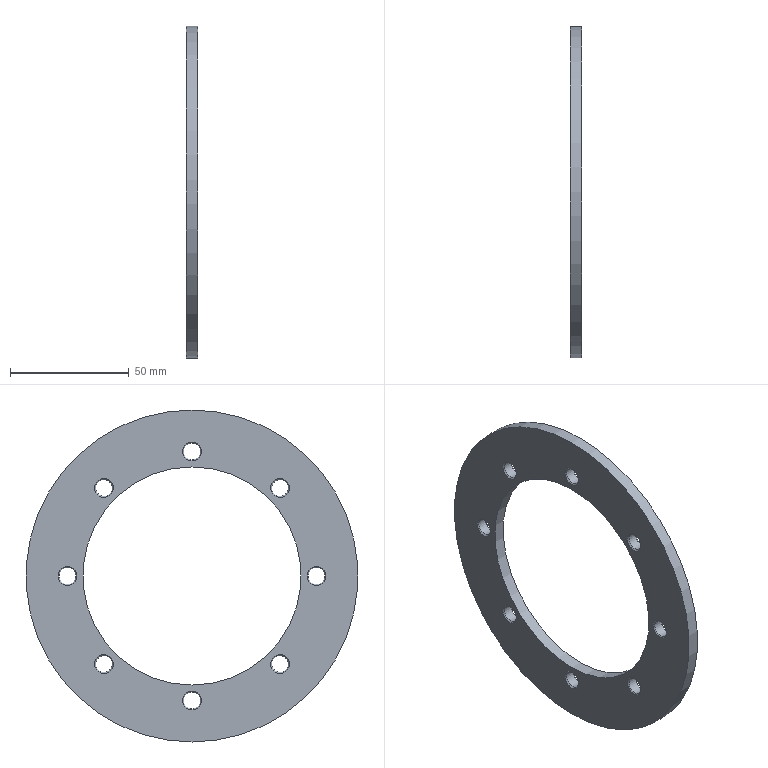Part | STEP file | Brake stopper | 1 solid | 28 faces | box 5 x 140 x 140 mm | volume 42146 mm3 | cone 16 | cylinder 10 | plane 2 | commonest cylinder face diameters 7 x8 92 x1 140 x1
STEP:
#1=CARTESIAN_POINT('',(0.,0.,-70.));
#2=VERTEX_POINT('',#1);
#3=CARTESIAN_POINT('',(0.,0.,0.));
#4=DIRECTION('',(1.,0.,0.));
#5=DIRECTION('',(0.,0.,-1.));
#6=AXIS2_PLACEMENT_3D('',#3,#4,#5);
#7=CIRCLE('',#6,70.);
#8=EDGE_CURVE('',#2,#2,#7,.T.);
#9=ORIENTED_EDGE('',*,*,#8,.F.);
#10=EDGE_LOOP('',(#9));
#11=FACE_BOUND('',#10,.T.);
#12=CARTESIAN_POINT('',(0.,39.952,34.295));
#13=VERTEX_POINT('',#12);
#14=CARTESIAN_POINT('',(0.,37.123,37.123));
#15=DIRECTION('',(-1.,0.,0.));
#16=DIRECTION('',(0.,0.7071,-0.7071));
#17=AXIS2_PLACEMENT_3D('',#14,#15,#16);
#18=CIRCLE('',#17,4.);
#19=EDGE_CURVE('',#13,#13,#18,.F.);
#20=ORIENTED_EDGE('',*,*,#19,.T.);
#21=EDGE_LOOP('',(#20));
#22=FACE_BOUND('',#21,.T.);
#23=CARTESIAN_POINT('',(0.,34.295,-39.952));
#24=VERTEX_POINT('',#23);
#25=CARTESIAN_POINT('',(0.,37.123,-37.123));
#26=DIRECTION('',(-1.,0.,0.));
#27=DIRECTION('',(0.,-0.7071,-0.7071));
#28=AXIS2_PLACEMENT_3D('',#25,#26,#27);
#29=CIRCLE('',#28,4.);
#30=EDGE_CURVE('',#24,#24,#29,.F.);
#31=ORIENTED_EDGE('',*,*,#30,.T.);
#32=EDGE_LOOP('',(#31));
#33=FACE_BOUND('',#32,.T.);
#34=CARTESIAN_POINT('',(0.,-39.952,-34.295));
#35=VERTEX_POINT('',#34);
#36=CARTESIAN_POINT('',(0.,-37.123,-37.123));
#37=DIRECTION('',(-1.,0.,0.));
#38=DIRECTION('',(0.,-0.7071,0.7071));
#39=AXIS2_PLACEMENT_3D('',#36,#37,#38);
#40=CIRCLE('',#39,4.);
#41=EDGE_CURVE('',#35,#35,#40,.F.);
#42=ORIENTED_EDGE('',*,*,#41,.T.);
#43=EDGE_LOOP('',(#42));
#44=FACE_BOUND('',#43,.T.);
#45=CARTESIAN_POINT('',(0.,-34.295,39.952));
#46=VERTEX_POINT('',#45);
#47=CARTESIAN_POINT('',(0.,-37.123,37.123));
#48=DIRECTION('',(-1.,0.,0.));
#49=DIRECTION('',(0.,0.7071,0.7071));
#50=AXIS2_PLACEMENT_3D('',#47,#48,#49);
#51=CIRCLE('',#50,4.);
#52=EDGE_CURVE('',#46,#46,#51,.F.);
#53=ORIENTED_EDGE('',*,*,#52,.T.);
#54=EDGE_LOOP('',(#53));
#55=FACE_BOUND('',#54,.T.);
#56=CARTESIAN_POINT('',(0.,4.,52.5));
#57=VERTEX_POINT('',#56);
#58=CARTESIAN_POINT('',(0.,0.,52.5));
#59=DIRECTION('',(-1.,0.,0.));
#60=DIRECTION('',(0.,1.,0.));
#61=AXIS2_PLACEMENT_3D('',#58,#59,#60);
#62=CIRCLE('',#61,4.);
#63=EDGE_CURVE('',#57,#57,#62,.F.);
#64=ORIENTED_EDGE('',*,*,#63,.T.);
#65=EDGE_LOOP('',(#64));
#66=FACE_BOUND('',#65,.T.);
#67=CARTESIAN_POINT('',(0.,0.,-46.));
#68=VERTEX_POINT('',#67);
#69=CARTESIAN_POINT('',(0.,0.,0.));
#70=DIRECTION('',(1.,0.,0.));
#71=DIRECTION('',(0.,0.,-1.));
#72=AXIS2_PLACEMENT_3D('',#69,#70,#71);
#73=CIRCLE('',#72,46.);
#74=EDGE_CURVE('',#68,#68,#73,.T.);
#75=ORIENTED_EDGE('',*,*,#74,.T.);
#76=EDGE_LOOP('',(#75));
#77=FACE_BOUND('',#76,.T.);
#78=CARTESIAN_POINT('',(0.,-52.5,4.));
#79=VERTEX_POINT('',#78);
#80=CARTESIAN_POINT('',(0.,-52.5,0.));
#81=DIRECTION('',(-1.,0.,0.));
#82=DIRECTION('',(0.,0.,1.));
#83=AXIS2_PLACEMENT_3D('',#80,#81,#82);
#84=CIRCLE('',#83,4.);
#85=EDGE_CURVE('',#79,#79,#84,.F.);
#86=ORIENTED_EDGE('',*,*,#85,.T.);
#87=EDGE_LOOP('',(#86));
#88=FACE_BOUND('',#87,.T.);
#89=CARTESIAN_POINT('',(0.,-4.,-52.5));
#90=VERTEX_POINT('',#89);
#91=CARTESIAN_POINT('',(0.,0.,-52.5));
#92=DIRECTION('',(-1.,0.,0.));
#93=DIRECTION('',(0.,-1.,0.));
#94=AXIS2_PLACEMENT_3D('',#91,#92,#93);
#95=CIRCLE('',#94,4.);
#96=EDGE_CURVE('',#90,#90,#95,.F.);
#97=ORIENTED_EDGE('',*,*,#96,.T.);
#98=EDGE_LOOP('',(#97));
#99=FACE_BOUND('',#98,.T.);
#100=CARTESIAN_POINT('',(0.,52.5,-4.));
#101=VERTEX_POINT('',#100);
#102=CARTESIAN_POINT('',(0.,52.5,0.));
#103=DIRECTION('',(-1.,0.,0.));
#104=DIRECTION('',(0.,0.,-1.));
#105=AXIS2_PLACEMENT_3D('',#102,#103,#104);
#106=CIRCLE('',#105,4.);
#107=EDGE_CURVE('',#101,#101,#106,.F.);
#108=ORIENTED_EDGE('',*,*,#107,.T.);
#109=EDGE_LOOP('',(#108));
#110=FACE_BOUND('',#109,.T.);
#111=CARTESIAN_POINT('',(0.,0.,0.));
#112=DIRECTION('',(1.,0.,0.));
#113=DIRECTION('',(0.,0.,-1.));
#114=AXIS2_PLACEMENT_3D('',#111,#112,#113);
#115=PLANE('',#114);
#116=ADVANCED_FACE('',(#11,#22,#33,#44,#55,#66,#77,#88,#99,#110),#115,.F.);
#117=CARTESIAN_POINT('',(5.,0.,-70.));
#118=VERTEX_POINT('',#117);
#119=CARTESIAN_POINT('',(5.,0.,0.));
#120=DIRECTION('',(1.,0.,0.));
#121=DIRECTION('',(0.,0.,-1.));
#122=AXIS2_PLACEMENT_3D('',#119,#120,#121);
#123=CIRCLE('',#122,70.);
#124=EDGE_CURVE('',#118,#118,#123,.T.);
#125=ORIENTED_EDGE('',*,*,#124,.T.);
#126=EDGE_LOOP('',(#125));
#127=FACE_BOUND('',#126,.T.);
#128=CARTESIAN_POINT('',(5.,39.952,34.295));
#129=VERTEX_POINT('',#128);
#130=CARTESIAN_POINT('',(5.,37.123,37.123));
#131=DIRECTION('',(-1.,0.,0.));
#132=DIRECTION('',(0.,0.7071,-0.7071));
#133=AXIS2_PLACEMENT_3D('',#130,#131,#132);
#134=CIRCLE('',#133,4.);
#135=EDGE_CURVE('',#129,#129,#134,.T.);
#136=ORIENTED_EDGE('',*,*,#135,.T.);
#137=EDGE_LOOP('',(#136));
#138=FACE_BOUND('',#137,.T.);
#139=CARTESIAN_POINT('',(5.,34.295,-39.952));
#140=VERTEX_POINT('',#139);
#141=CARTESIAN_POINT('',(5.,37.123,-37.123));
#142=DIRECTION('',(-1.,0.,0.));
#143=DIRECTION('',(0.,-0.7071,-0.7071));
#144=AXIS2_PLACEMENT_3D('',#141,#142,#143);
#145=CIRCLE('',#144,4.);
#146=EDGE_CURVE('',#140,#140,#145,.T.);
#147=ORIENTED_EDGE('',*,*,#146,.T.);
#148=EDGE_LOOP('',(#147));
#149=FACE_BOUND('',#148,.T.);
#150=CARTESIAN_POINT('',(5.,-39.952,-34.295));
#151=VERTEX_POINT('',#150);
#152=CARTESIAN_POINT('',(5.,-37.123,-37.123));
#153=DIRECTION('',(-1.,0.,0.));
#154=DIRECTION('',(0.,-0.7071,0.7071));
#155=AXIS2_PLACEMENT_3D('',#152,#153,#154);
#156=CIRCLE('',#155,4.);
#157=EDGE_CURVE('',#151,#151,#156,.T.);
#158=ORIENTED_EDGE('',*,*,#157,.T.);
#159=EDGE_LOOP('',(#158));
#160=FACE_BOUND('',#159,.T.);
#161=CARTESIAN_POINT('',(5.,-34.295,39.952));
#162=VERTEX_POINT('',#161);
#163=CARTESIAN_POINT('',(5.,-37.123,37.123));
#164=DIRECTION('',(-1.,0.,0.));
#165=DIRECTION('',(0.,0.7071,0.7071));
#166=AXIS2_PLACEMENT_3D('',#163,#164,#165);
#167=CIRCLE('',#166,4.);
#168=EDGE_CURVE('',#162,#162,#167,.T.);
#169=ORIENTED_EDGE('',*,*,#168,.T.);
#170=EDGE_LOOP('',(#169));
#171=FACE_BOUND('',#170,.T.);
#172=CARTESIAN_POINT('',(5.,4.,52.5));
#173=VERTEX_POINT('',#172);
#174=CARTESIAN_POINT('',(5.,0.,52.5));
#175=DIRECTION('',(-1.,0.,0.));
#176=DIRECTION('',(0.,1.,0.));
#177=AXIS2_PLACEMENT_3D('',#174,#175,#176);
#178=CIRCLE('',#177,4.);
#179=EDGE_CURVE('',#173,#173,#178,.T.);
#180=ORIENTED_EDGE('',*,*,#179,.T.);
#181=EDGE_LOOP('',(#180));
#182=FACE_BOUND('',#181,.T.);
#183=CARTESIAN_POINT('',(5.,0.,-46.));
#184=VERTEX_POINT('',#183);
#185=CARTESIAN_POINT('',(5.,0.,0.));
#186=DIRECTION('',(1.,0.,0.));
#187=DIRECTION('',(0.,0.,-1.));
#188=AXIS2_PLACEMENT_3D('',#185,#186,#187);
#189=CIRCLE('',#188,46.);
#190=EDGE_CURVE('',#184,#184,#189,.F.);
#191=ORIENTED_EDGE('',*,*,#190,.T.);
#192=EDGE_LOOP('',(#191));
#193=FACE_BOUND('',#192,.T.);
#194=CARTESIAN_POINT('',(5.,-52.5,4.));
#195=VERTEX_POINT('',#194);
#196=CARTESIAN_POINT('',(5.,-52.5,0.));
#197=DIRECTION('',(-1.,0.,0.));
#198=DIRECTION('',(0.,0.,1.));
#199=AXIS2_PLACEMENT_3D('',#196,#197,#198);
#200=CIRCLE('',#199,4.);
#201=EDGE_CURVE('',#195,#195,#200,.T.);
#202=ORIENTED_EDGE('',*,*,#201,.T.);
#203=EDGE_LOOP('',(#202));
#204=FACE_BOUND('',#203,.T.);
#205=CARTESIAN_POINT('',(5.,-4.,-52.5));
#206=VERTEX_POINT('',#205);
#207=CARTESIAN_POINT('',(5.,0.,-52.5));
#208=DIRECTION('',(-1.,0.,0.));
#209=DIRECTION('',(0.,-1.,0.));
#210=AXIS2_PLACEMENT_3D('',#207,#208,#209);
#211=CIRCLE('',#210,4.);
#212=EDGE_CURVE('',#206,#206,#211,.T.);
#213=ORIENTED_EDGE('',*,*,#212,.T.);
#214=EDGE_LOOP('',(#213));
#215=FACE_BOUND('',#214,.T.);
#216=CARTESIAN_POINT('',(5.,52.5,-4.));
#217=VERTEX_POINT('',#216);
#218=CARTESIAN_POINT('',(5.,52.5,0.));
#219=DIRECTION('',(-1.,0.,0.));
#220=DIRECTION('',(0.,0.,-1.));
#221=AXIS2_PLACEMENT_3D('',#218,#219,#220);
#222=CIRCLE('',#221,4.);
#223=EDGE_CURVE('',#217,#217,#222,.T.);
#224=ORIENTED_EDGE('',*,*,#223,.T.);
#225=EDGE_LOOP('',(#224));
#226=FACE_BOUND('',#225,.T.);
#227=CARTESIAN_POINT('',(5.,0.,0.));
#228=DIRECTION('',(1.,0.,0.));
#229=DIRECTION('',(0.,0.,-1.));
#230=AXIS2_PLACEMENT_3D('',#227,#228,#229);
#231=PLANE('',#230);
#232=ADVANCED_FACE('',(#127,#138,#149,#160,#171,#182,#193,#204,#215,#226),#231,.T.);
#233=CARTESIAN_POINT('',(4.5,39.598,34.648));
#234=VERTEX_POINT('',#233);
#235=CARTESIAN_POINT('',(4.5,37.123,37.123));
#236=DIRECTION('',(-1.,0.,0.));
#237=DIRECTION('',(0.,0.7071,-0.7071));
#238=AXIS2_PLACEMENT_3D('',#235,#236,#237);
#239=CIRCLE('',#238,3.5);
#240=EDGE_CURVE('',#234,#234,#239,.T.);
#241=ORIENTED_EDGE('',*,*,#240,.F.);
#242=EDGE_LOOP('',(#241));
#243=FACE_OUTER_BOUND('',#242,.T.);
#244=CARTESIAN_POINT('',(0.5,39.598,34.648));
#245=VERTEX_POINT('',#244);
#246=CARTESIAN_POINT('',(0.5,37.123,37.123));
#247=DIRECTION('',(-1.,0.,0.));
#248=DIRECTION('',(0.,0.7071,-0.7071));
#249=AXIS2_PLACEMENT_3D('',#246,#247,#248);
#250=CIRCLE('',#249,3.5);
#251=EDGE_CURVE('',#245,#245,#250,.F.);
#252=ORIENTED_EDGE('',*,*,#251,.F.);
#253=EDGE_LOOP('',(#252));
#254=FACE_OUTER_BOUND('',#253,.T.);
#255=CARTESIAN_POINT('',(40.,37.123,37.123));
#256=DIRECTION('',(-1.,0.,0.));
#257=DIRECTION('',(0.,0.7071,-0.7071));
#258=AXIS2_PLACEMENT_3D('',#255,#256,#257);
#259=CYLINDRICAL_SURFACE('',#258,3.5);
#260=ADVANCED_FACE('',(#243,#254),#259,.F.);
#261=CARTESIAN_POINT('',(4.5,52.5,-3.5));
#262=VERTEX_POINT('',#261);
#263=CARTESIAN_POINT('',(4.5,52.5,0.));
#264=DIRECTION('',(-1.,0.,0.));
#265=DIRECTION('',(0.,0.,-1.));
#266=AXIS2_PLACEMENT_3D('',#263,#264,#265);
#267=CIRCLE('',#266,3.5);
#268=EDGE_CURVE('',#262,#262,#267,.T.);
#269=ORIENTED_EDGE('',*,*,#268,.F.);
#270=EDGE_LOOP('',(#269));
#271=FACE_OUTER_BOUND('',#270,.T.);
#272=CARTESIAN_POINT('',(0.5,52.5,-3.5));
#273=VERTEX_POINT('',#272);
#274=CARTESIAN_POINT('',(0.5,52.5,0.));
#275=DIRECTION('',(-1.,0.,0.));
#276=DIRECTION('',(0.,0.,-1.));
#277=AXIS2_PLACEMENT_3D('',#274,#275,#276);
#278=CIRCLE('',#277,3.5);
#279=EDGE_CURVE('',#273,#273,#278,.F.);
#280=ORIENTED_EDGE('',*,*,#279,.F.);
#281=EDGE_LOOP('',(#280));
#282=FACE_OUTER_BOUND('',#281,.T.);
#283=CARTESIAN_POINT('',(40.,52.5,0.));
#284=DIRECTION('',(-1.,0.,0.));
#285=DIRECTION('',(0.,0.,-1.));
#286=AXIS2_PLACEMENT_3D('',#283,#284,#285);
#287=CYLINDRICAL_SURFACE('',#286,3.5);
#288=ADVANCED_FACE('',(#271,#282),#287,.F.);
#289=CARTESIAN_POINT('',(4.5,34.648,-39.598));
#290=VERTEX_POINT('',#289);
#291=CARTESIAN_POINT('',(4.5,37.123,-37.123));
#292=DIRECTION('',(-1.,0.,0.));
#293=DIRECTION('',(0.,-0.7071,-0.7071));
#294=AXIS2_PLACEMENT_3D('',#291,#292,#293);
#295=CIRCLE('',#294,3.5);
#296=EDGE_CURVE('',#290,#290,#295,.T.);
#297=ORIENTED_EDGE('',*,*,#296,.F.);
#298=EDGE_LOOP('',(#297));
#299=FACE_OUTER_BOUND('',#298,.T.);
#300=CARTESIAN_POINT('',(0.5,34.648,-39.598));
#301=VERTEX_POINT('',#300);
#302=CARTESIAN_POINT('',(0.5,37.123,-37.123));
#303=DIRECTION('',(-1.,0.,0.));
#304=DIRECTION('',(0.,-0.7071,-0.7071));
#305=AXIS2_PLACEMENT_3D('',#302,#303,#304);
#306=CIRCLE('',#305,3.5);
#307=EDGE_CURVE('',#301,#301,#306,.F.);
#308=ORIENTED_EDGE('',*,*,#307,.F.);
#309=EDGE_LOOP('',(#308));
#310=FACE_OUTER_BOUND('',#309,.T.);
#311=CARTESIAN_POINT('',(40.,37.123,-37.123));
#312=DIRECTION('',(-1.,0.,0.));
#313=DIRECTION('',(0.,-0.7071,-0.7071));
#314=AXIS2_PLACEMENT_3D('',#311,#312,#313);
#315=CYLINDRICAL_SURFACE('',#314,3.5);
#316=ADVANCED_FACE('',(#299,#310),#315,.F.);
#317=CARTESIAN_POINT('',(4.5,-3.5,-52.5));
#318=VERTEX_POINT('',#317);
#319=CARTESIAN_POINT('',(4.5,0.,-52.5));
#320=DIRECTION('',(-1.,0.,0.));
#321=DIRECTION('',(0.,-1.,0.));
#322=AXIS2_PLACEMENT_3D('',#319,#320,#321);
#323=CIRCLE('',#322,3.5);
#324=EDGE_CURVE('',#318,#318,#323,.T.);
#325=ORIENTED_EDGE('',*,*,#324,.F.);
#326=EDGE_LOOP('',(#325));
#327=FACE_OUTER_BOUND('',#326,.T.);
#328=CARTESIAN_POINT('',(0.5,-3.5,-52.5));
#329=VERTEX_POINT('',#328);
#330=CARTESIAN_POINT('',(0.5,0.,-52.5));
#331=DIRECTION('',(-1.,0.,0.));
#332=DIRECTION('',(0.,-1.,0.));
#333=AXIS2_PLACEMENT_3D('',#330,#331,#332);
#334=CIRCLE('',#333,3.5);
#335=EDGE_CURVE('',#329,#329,#334,.F.);
#336=ORIENTED_EDGE('',*,*,#335,.F.);
#337=EDGE_LOOP('',(#336));
#338=FACE_OUTER_BOUND('',#337,.T.);
#339=CARTESIAN_POINT('',(40.,0.,-52.5));
#340=DIRECTION('',(-1.,0.,0.));
#341=DIRECTION('',(0.,-1.,0.));
#342=AXIS2_PLACEMENT_3D('',#339,#340,#341);
#343=CYLINDRICAL_SURFACE('',#342,3.5);
#344=ADVANCED_FACE('',(#327,#338),#343,.F.);
#345=CARTESIAN_POINT('',(4.5,-39.598,-34.648));
#346=VERTEX_POINT('',#345);
#347=CARTESIAN_POINT('',(4.5,-37.123,-37.123));
#348=DIRECTION('',(-1.,0.,0.));
#349=DIRECTION('',(0.,-0.7071,0.7071));
#350=AXIS2_PLACEMENT_3D('',#347,#348,#349);
#351=CIRCLE('',#350,3.5);
#352=EDGE_CURVE('',#346,#346,#351,.T.);
#353=ORIENTED_EDGE('',*,*,#352,.F.);
#354=EDGE_LOOP('',(#353));
#355=FACE_OUTER_BOUND('',#354,.T.);
#356=CARTESIAN_POINT('',(0.5,-39.598,-34.648));
#357=VERTEX_POINT('',#356);
#358=CARTESIAN_POINT('',(0.5,-37.123,-37.123));
#359=DIRECTION('',(-1.,0.,0.));
#360=DIRECTION('',(0.,-0.7071,0.7071));
#361=AXIS2_PLACEMENT_3D('',#358,#359,#360);
#362=CIRCLE('',#361,3.5);
#363=EDGE_CURVE('',#357,#357,#362,.F.);
#364=ORIENTED_EDGE('',*,*,#363,.F.);
#365=EDGE_LOOP('',(#364));
#366=FACE_OUTER_BOUND('',#365,.T.);
#367=CARTESIAN_POINT('',(40.,-37.123,-37.123));
#368=DIRECTION('',(-1.,0.,0.));
#369=DIRECTION('',(0.,-0.7071,0.7071));
#370=AXIS2_PLACEMENT_3D('',#367,#368,#369);
#371=CYLINDRICAL_SURFACE('',#370,3.5);
#372=ADVANCED_FACE('',(#355,#366),#371,.F.);
#373=CARTESIAN_POINT('',(4.5,-52.5,3.5));
#374=VERTEX_POINT('',#373);
#375=CARTESIAN_POINT('',(4.5,-52.5,0.));
#376=DIRECTION('',(-1.,0.,0.));
#377=DIRECTION('',(0.,0.,1.));
#378=AXIS2_PLACEMENT_3D('',#375,#376,#377);
#379=CIRCLE('',#378,3.5);
#380=EDGE_CURVE('',#374,#374,#379,.T.);
#381=ORIENTED_EDGE('',*,*,#380,.F.);
#382=EDGE_LOOP('',(#381));
#383=FACE_OUTER_BOUND('',#382,.T.);
#384=CARTESIAN_POINT('',(0.5,-52.5,3.5));
#385=VERTEX_POINT('',#384);
#386=CARTESIAN_POINT('',(0.5,-52.5,0.));
#387=DIRECTION('',(-1.,0.,0.));
#388=DIRECTION('',(0.,0.,1.));
#389=AXIS2_PLACEMENT_3D('',#386,#387,#388);
#390=CIRCLE('',#389,3.5);
#391=EDGE_CURVE('',#385,#385,#390,.F.);
#392=ORIENTED_EDGE('',*,*,#391,.F.);
#393=EDGE_LOOP('',(#392));
#394=FACE_OUTER_BOUND('',#393,.T.);
#395=CARTESIAN_POINT('',(40.,-52.5,0.));
#396=DIRECTION('',(-1.,0.,0.));
#397=DIRECTION('',(0.,0.,1.));
#398=AXIS2_PLACEMENT_3D('',#395,#396,#397);
#399=CYLINDRICAL_SURFACE('',#398,3.5);
#400=ADVANCED_FACE('',(#383,#394),#399,.F.);
#401=CARTESIAN_POINT('',(4.5,-34.648,39.598));
#402=VERTEX_POINT('',#401);
#403=CARTESIAN_POINT('',(4.5,-37.123,37.123));
#404=DIRECTION('',(-1.,0.,0.));
#405=DIRECTION('',(0.,0.7071,0.7071));
#406=AXIS2_PLACEMENT_3D('',#403,#404,#405);
#407=CIRCLE('',#406,3.5);
#408=EDGE_CURVE('',#402,#402,#407,.T.);
#409=ORIENTED_EDGE('',*,*,#408,.F.);
#410=EDGE_LOOP('',(#409));
#411=FACE_OUTER_BOUND('',#410,.T.);
#412=CARTESIAN_POINT('',(0.5,-34.648,39.598));
#413=VERTEX_POINT('',#412);
#414=CARTESIAN_POINT('',(0.5,-37.123,37.123));
#415=DIRECTION('',(-1.,0.,0.));
#416=DIRECTION('',(0.,0.7071,0.7071));
#417=AXIS2_PLACEMENT_3D('',#414,#415,#416);
#418=CIRCLE('',#417,3.5);
#419=EDGE_CURVE('',#413,#413,#418,.F.);
#420=ORIENTED_EDGE('',*,*,#419,.F.);
#421=EDGE_LOOP('',(#420));
#422=FACE_OUTER_BOUND('',#421,.T.);
#423=CARTESIAN_POINT('',(40.,-37.123,37.123));
#424=DIRECTION('',(-1.,0.,0.));
#425=DIRECTION('',(0.,0.7071,0.7071));
#426=AXIS2_PLACEMENT_3D('',#423,#424,#425);
#427=CYLINDRICAL_SURFACE('',#426,3.5);
#428=ADVANCED_FACE('',(#411,#422),#427,.F.);
#429=ORIENTED_EDGE('',*,*,#124,.F.);
#430=EDGE_LOOP('',(#429));
#431=FACE_OUTER_BOUND('',#430,.T.);
#432=ORIENTED_EDGE('',*,*,#8,.T.);
#433=EDGE_LOOP('',(#432));
#434=FACE_OUTER_BOUND('',#433,.T.);
#435=CARTESIAN_POINT('',(0.,0.,0.));
#436=DIRECTION('',(1.,0.,0.));
#437=DIRECTION('',(0.,0.,-1.));
#438=AXIS2_PLACEMENT_3D('',#435,#436,#437);
#439=CYLINDRICAL_SURFACE('',#438,70.);
#440=ADVANCED_FACE('',(#431,#434),#439,.T.);
#441=ORIENTED_EDGE('',*,*,#190,.F.);
#442=EDGE_LOOP('',(#441));
#443=FACE_OUTER_BOUND('',#442,.T.);
#444=ORIENTED_EDGE('',*,*,#74,.F.);
#445=EDGE_LOOP('',(#444));
#446=FACE_OUTER_BOUND('',#445,.T.);
#447=CARTESIAN_POINT('',(0.,0.,0.));
#448=DIRECTION('',(1.,0.,0.));
#449=DIRECTION('',(0.,0.,-1.));
#450=AXIS2_PLACEMENT_3D('',#447,#448,#449);
#451=CYLINDRICAL_SURFACE('',#450,46.);
#452=ADVANCED_FACE('',(#443,#446),#451,.F.);
#453=CARTESIAN_POINT('',(0.5,3.5,52.5));
#454=VERTEX_POINT('',#453);
#455=CARTESIAN_POINT('',(0.5,0.,52.5));
#456=DIRECTION('',(-1.,0.,0.));
#457=DIRECTION('',(0.,1.,0.));
#458=AXIS2_PLACEMENT_3D('',#455,#456,#457);
#459=CIRCLE('',#458,3.5);
#460=EDGE_CURVE('',#454,#454,#459,.F.);
#461=ORIENTED_EDGE('',*,*,#460,.T.);
#462=EDGE_LOOP('',(#461));
#463=FACE_OUTER_BOUND('',#462,.T.);
#464=ORIENTED_EDGE('',*,*,#63,.F.);
#465=EDGE_LOOP('',(#464));
#466=FACE_OUTER_BOUND('',#465,.T.);
#467=CARTESIAN_POINT('',(0.25,0.,52.5));
#468=DIRECTION('',(-1.,0.,0.));
#469=DIRECTION('',(0.,1.,0.));
#470=AXIS2_PLACEMENT_3D('',#467,#468,#469);
#471=CONICAL_SURFACE('',#470,3.75,0.7854);
#472=ADVANCED_FACE('',(#463,#466),#471,.F.);
#473=ORIENTED_EDGE('',*,*,#179,.F.);
#474=EDGE_LOOP('',(#473));
#475=FACE_OUTER_BOUND('',#474,.T.);
#476=CARTESIAN_POINT('',(4.5,3.5,52.5));
#477=VERTEX_POINT('',#476);
#478=CARTESIAN_POINT('',(4.5,0.,52.5));
#479=DIRECTION('',(-1.,0.,0.));
#480=DIRECTION('',(0.,1.,0.));
#481=AXIS2_PLACEMENT_3D('',#478,#479,#480);
#482=CIRCLE('',#481,3.5);
#483=EDGE_CURVE('',#477,#477,#482,.T.);
#484=ORIENTED_EDGE('',*,*,#483,.T.);
#485=EDGE_LOOP('',(#484));
#486=FACE_OUTER_BOUND('',#485,.T.);
#487=CARTESIAN_POINT('',(4.75,0.,52.5));
#488=DIRECTION('',(1.,0.,0.));
#489=DIRECTION('',(0.,-1.,0.));
#490=AXIS2_PLACEMENT_3D('',#487,#488,#489);
#491=CONICAL_SURFACE('',#490,3.75,0.7854);
#492=ADVANCED_FACE('',(#475,#486),#491,.F.);
#493=ORIENTED_EDGE('',*,*,#483,.F.);
#494=EDGE_LOOP('',(#493));
#495=FACE_OUTER_BOUND('',#494,.T.);
#496=ORIENTED_EDGE('',*,*,#460,.F.);
#497=EDGE_LOOP('',(#496));
#498=FACE_OUTER_BOUND('',#497,.T.);
#499=CARTESIAN_POINT('',(40.,0.,52.5));
#500=DIRECTION('',(-1.,0.,0.));
#501=DIRECTION('',(0.,1.,0.));
#502=AXIS2_PLACEMENT_3D('',#499,#500,#501);
#503=CYLINDRICAL_SURFACE('',#502,3.5);
#504=ADVANCED_FACE('',(#495,#498),#503,.F.);
#505=ORIENTED_EDGE('',*,*,#419,.T.);
#506=EDGE_LOOP('',(#505));
#507=FACE_OUTER_BOUND('',#506,.T.);
#508=ORIENTED_EDGE('',*,*,#52,.F.);
#509=EDGE_LOOP('',(#508));
#510=FACE_OUTER_BOUND('',#509,.T.);
#511=CARTESIAN_POINT('',(0.25,-37.123,37.123));
#512=DIRECTION('',(-1.,0.,0.));
#513=DIRECTION('',(0.,0.7071,0.7071));
#514=AXIS2_PLACEMENT_3D('',#511,#512,#513);
#515=CONICAL_SURFACE('',#514,3.75,0.7854);
#516=ADVANCED_FACE('',(#507,#510),#515,.F.);
#517=ORIENTED_EDGE('',*,*,#168,.F.);
#518=EDGE_LOOP('',(#517));
#519=FACE_OUTER_BOUND('',#518,.T.);
#520=ORIENTED_EDGE('',*,*,#408,.T.);
#521=EDGE_LOOP('',(#520));
#522=FACE_OUTER_BOUND('',#521,.T.);
#523=CARTESIAN_POINT('',(4.75,-37.123,37.123));
#524=DIRECTION('',(1.,0.,0.));
#525=DIRECTION('',(0.,-0.7071,-0.7071));
#526=AXIS2_PLACEMENT_3D('',#523,#524,#525);
#527=CONICAL_SURFACE('',#526,3.75,0.7854);
#528=ADVANCED_FACE('',(#519,#522),#527,.F.);
#529=ORIENTED_EDGE('',*,*,#391,.T.);
#530=EDGE_LOOP('',(#529));
#531=FACE_OUTER_BOUND('',#530,.T.);
#532=ORIENTED_EDGE('',*,*,#85,.F.);
#533=EDGE_LOOP('',(#532));
#534=FACE_OUTER_BOUND('',#533,.T.);
#535=CARTESIAN_POINT('',(0.25,-52.5,0.));
#536=DIRECTION('',(-1.,0.,0.));
#537=DIRECTION('',(0.,0.,1.));
#538=AXIS2_PLACEMENT_3D('',#535,#536,#537);
#539=CONICAL_SURFACE('',#538,3.75,0.7854);
#540=ADVANCED_FACE('',(#531,#534),#539,.F.);
#541=ORIENTED_EDGE('',*,*,#201,.F.);
#542=EDGE_LOOP('',(#541));
#543=FACE_OUTER_BOUND('',#542,.T.);
#544=ORIENTED_EDGE('',*,*,#380,.T.);
#545=EDGE_LOOP('',(#544));
#546=FACE_OUTER_BOUND('',#545,.T.);
#547=CARTESIAN_POINT('',(4.75,-52.5,0.));
#548=DIRECTION('',(1.,0.,0.));
#549=DIRECTION('',(0.,0.,-1.));
#550=AXIS2_PLACEMENT_3D('',#547,#548,#549);
#551=CONICAL_SURFACE('',#550,3.75,0.7854);
#552=ADVANCED_FACE('',(#543,#546),#551,.F.);
#553=ORIENTED_EDGE('',*,*,#363,.T.);
#554=EDGE_LOOP('',(#553));
#555=FACE_OUTER_BOUND('',#554,.T.);
#556=ORIENTED_EDGE('',*,*,#41,.F.);
#557=EDGE_LOOP('',(#556));
#558=FACE_OUTER_BOUND('',#557,.T.);
#559=CARTESIAN_POINT('',(0.25,-37.123,-37.123));
#560=DIRECTION('',(-1.,0.,0.));
#561=DIRECTION('',(0.,-0.7071,0.7071));
#562=AXIS2_PLACEMENT_3D('',#559,#560,#561);
#563=CONICAL_SURFACE('',#562,3.75,0.7854);
#564=ADVANCED_FACE('',(#555,#558),#563,.F.);
#565=ORIENTED_EDGE('',*,*,#157,.F.);
#566=EDGE_LOOP('',(#565));
#567=FACE_OUTER_BOUND('',#566,.T.);
#568=ORIENTED_EDGE('',*,*,#352,.T.);
#569=EDGE_LOOP('',(#568));
#570=FACE_OUTER_BOUND('',#569,.T.);
#571=CARTESIAN_POINT('',(4.75,-37.123,-37.123));
#572=DIRECTION('',(1.,0.,0.));
#573=DIRECTION('',(0.,0.7071,-0.7071));
#574=AXIS2_PLACEMENT_3D('',#571,#572,#573);
#575=CONICAL_SURFACE('',#574,3.75,0.7854);
#576=ADVANCED_FACE('',(#567,#570),#575,.F.);
#577=ORIENTED_EDGE('',*,*,#335,.T.);
#578=EDGE_LOOP('',(#577));
#579=FACE_OUTER_BOUND('',#578,.T.);
#580=ORIENTED_EDGE('',*,*,#96,.F.);
#581=EDGE_LOOP('',(#580));
#582=FACE_OUTER_BOUND('',#581,.T.);
#583=CARTESIAN_POINT('',(0.25,0.,-52.5));
#584=DIRECTION('',(-1.,0.,0.));
#585=DIRECTION('',(0.,-1.,0.));
#586=AXIS2_PLACEMENT_3D('',#583,#584,#585);
#587=CONICAL_SURFACE('',#586,3.75,0.7854);
#588=ADVANCED_FACE('',(#579,#582),#587,.F.);
#589=ORIENTED_EDGE('',*,*,#212,.F.);
#590=EDGE_LOOP('',(#589));
#591=FACE_OUTER_BOUND('',#590,.T.);
#592=ORIENTED_EDGE('',*,*,#324,.T.);
#593=EDGE_LOOP('',(#592));
#594=FACE_OUTER_BOUND('',#593,.T.);
#595=CARTESIAN_POINT('',(4.75,0.,-52.5));
#596=DIRECTION('',(1.,0.,0.));
#597=DIRECTION('',(0.,1.,0.));
#598=AXIS2_PLACEMENT_3D('',#595,#596,#597);
#599=CONICAL_SURFACE('',#598,3.75,0.7854);
#600=ADVANCED_FACE('',(#591,#594),#599,.F.);
#601=ORIENTED_EDGE('',*,*,#307,.T.);
#602=EDGE_LOOP('',(#601));
#603=FACE_OUTER_BOUND('',#602,.T.);
#604=ORIENTED_EDGE('',*,*,#30,.F.);
#605=EDGE_LOOP('',(#604));
#606=FACE_OUTER_BOUND('',#605,.T.);
#607=CARTESIAN_POINT('',(0.25,37.123,-37.123));
#608=DIRECTION('',(-1.,0.,0.));
#609=DIRECTION('',(0.,-0.7071,-0.7071));
#610=AXIS2_PLACEMENT_3D('',#607,#608,#609);
#611=CONICAL_SURFACE('',#610,3.75,0.7854);
#612=ADVANCED_FACE('',(#603,#606),#611,.F.);
#613=ORIENTED_EDGE('',*,*,#146,.F.);
#614=EDGE_LOOP('',(#613));
#615=FACE_OUTER_BOUND('',#614,.T.);
#616=ORIENTED_EDGE('',*,*,#296,.T.);
#617=EDGE_LOOP('',(#616));
#618=FACE_OUTER_BOUND('',#617,.T.);
#619=CARTESIAN_POINT('',(4.75,37.123,-37.123));
#620=DIRECTION('',(1.,0.,0.));
#621=DIRECTION('',(0.,0.7071,0.7071));
#622=AXIS2_PLACEMENT_3D('',#619,#620,#621);
#623=CONICAL_SURFACE('',#622,3.75,0.7854);
#624=ADVANCED_FACE('',(#615,#618),#623,.F.);
#625=ORIENTED_EDGE('',*,*,#279,.T.);
#626=EDGE_LOOP('',(#625));
#627=FACE_OUTER_BOUND('',#626,.T.);
#628=ORIENTED_EDGE('',*,*,#107,.F.);
#629=EDGE_LOOP('',(#628));
#630=FACE_OUTER_BOUND('',#629,.T.);
#631=CARTESIAN_POINT('',(0.25,52.5,0.));
#632=DIRECTION('',(-1.,0.,0.));
#633=DIRECTION('',(0.,0.,-1.));
#634=AXIS2_PLACEMENT_3D('',#631,#632,#633);
#635=CONICAL_SURFACE('',#634,3.75,0.7854);
#636=ADVANCED_FACE('',(#627,#630),#635,.F.);
#637=ORIENTED_EDGE('',*,*,#223,.F.);
#638=EDGE_LOOP('',(#637));
#639=FACE_OUTER_BOUND('',#638,.T.);
#640=ORIENTED_EDGE('',*,*,#268,.T.);
#641=EDGE_LOOP('',(#640));
#642=FACE_OUTER_BOUND('',#641,.T.);
#643=CARTESIAN_POINT('',(4.75,52.5,0.));
#644=DIRECTION('',(1.,0.,0.));
#645=DIRECTION('',(0.,0.,1.));
#646=AXIS2_PLACEMENT_3D('',#643,#644,#645);
#647=CONICAL_SURFACE('',#646,3.75,0.7854);
#648=ADVANCED_FACE('',(#639,#642),#647,.F.);
#649=ORIENTED_EDGE('',*,*,#251,.T.);
#650=EDGE_LOOP('',(#649));
#651=FACE_OUTER_BOUND('',#650,.T.);
#652=ORIENTED_EDGE('',*,*,#19,.F.);
#653=EDGE_LOOP('',(#652));
#654=FACE_OUTER_BOUND('',#653,.T.);
#655=CARTESIAN_POINT('',(0.25,37.123,37.123));
#656=DIRECTION('',(-1.,0.,0.));
#657=DIRECTION('',(0.,0.7071,-0.7071));
#658=AXIS2_PLACEMENT_3D('',#655,#656,#657);
#659=CONICAL_SURFACE('',#658,3.75,0.7854);
#660=ADVANCED_FACE('',(#651,#654),#659,.F.);
#661=ORIENTED_EDGE('',*,*,#135,.F.);
#662=EDGE_LOOP('',(#661));
#663=FACE_OUTER_BOUND('',#662,.T.);
#664=ORIENTED_EDGE('',*,*,#240,.T.);
#665=EDGE_LOOP('',(#664));
#666=FACE_OUTER_BOUND('',#665,.T.);
#667=CARTESIAN_POINT('',(4.75,37.123,37.123));
#668=DIRECTION('',(1.,0.,0.));
#669=DIRECTION('',(0.,-0.7071,0.7071));
#670=AXIS2_PLACEMENT_3D('',#667,#668,#669);
#671=CONICAL_SURFACE('',#670,3.75,0.7854);
#672=ADVANCED_FACE('',(#663,#666),#671,.F.);
#673=CLOSED_SHELL('',(#116,#232,#260,#288,#316,#344,#372,#400,#428,#440,#452,#472,#492,#504,#516,#528,#540,#552,#564,#576,#588,#600,#612,#624,#636,#648,#660,#672));
#674=MANIFOLD_SOLID_BREP('',#673);
#675=(LENGTH_UNIT()NAMED_UNIT(*)SI_UNIT(.MILLI.,.METRE.));
#676=UNCERTAINTY_MEASURE_WITH_UNIT(LENGTH_MEASURE(0.00001),#675,'','');
#677=(NAMED_UNIT(*)PLANE_ANGLE_UNIT()SI_UNIT($,.RADIAN.));
#678=(NAMED_UNIT(*)SI_UNIT($,.STERADIAN.)SOLID_ANGLE_UNIT());
#679=(GEOMETRIC_REPRESENTATION_CONTEXT(3)GLOBAL_UNCERTAINTY_ASSIGNED_CONTEXT((#676))GLOBAL_UNIT_ASSIGNED_CONTEXT((#675,#677,#678))REPRESENTATION_CONTEXT('',''));
#680=ADVANCED_BREP_SHAPE_REPRESENTATION('',(#674),#679);